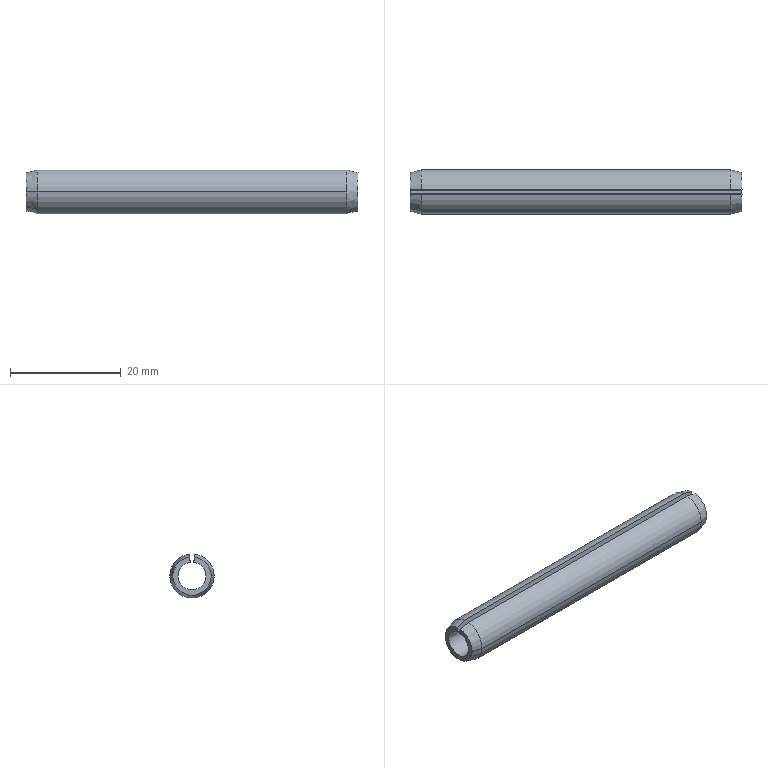Part | SolidWorks | features BaseBody 1 | 1 solid | 14 faces | box 60 x 8 x 7.968 mm | volume 1740 mm3 | cylinder 6 | cone 4 | plane 4 | commonest cylinder face diameters 5 x3 8 x3